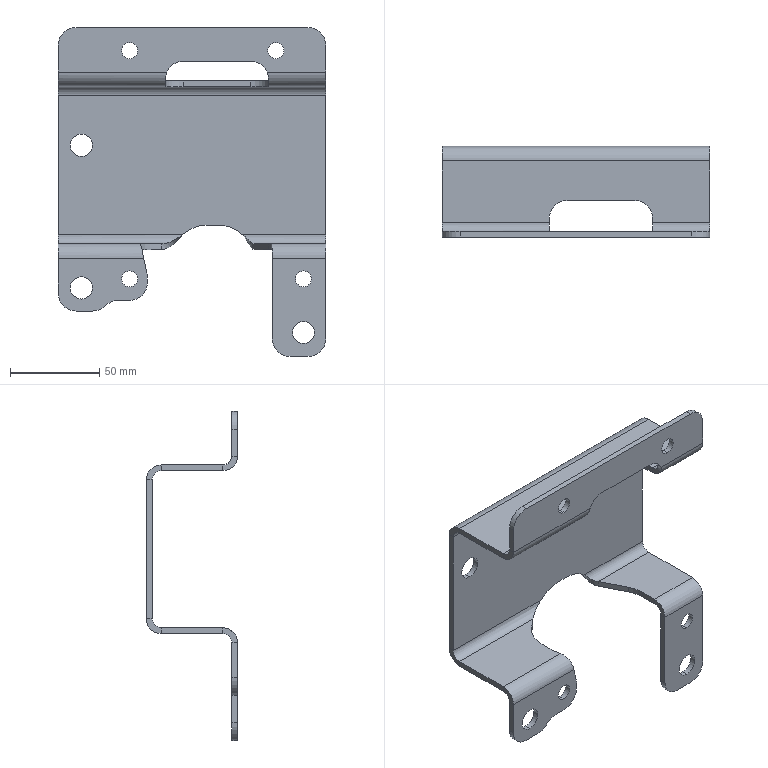Part | SolidWorks | features ICE 2, Fillet 1, FlatPattern 1, Fold 1, SMBaseFlange 1, SheetMetal 1, UnFold 1 | 1 solid | 106 faces | box 150 x 51 x 184.5 mm | volume 92629 mm3 | plane 54 | cylinder 46 | spline 6 | commonest cylinder face diameters 20 x12 9 x8 10 x7 16.4 x7 12.5 x6 40 x6